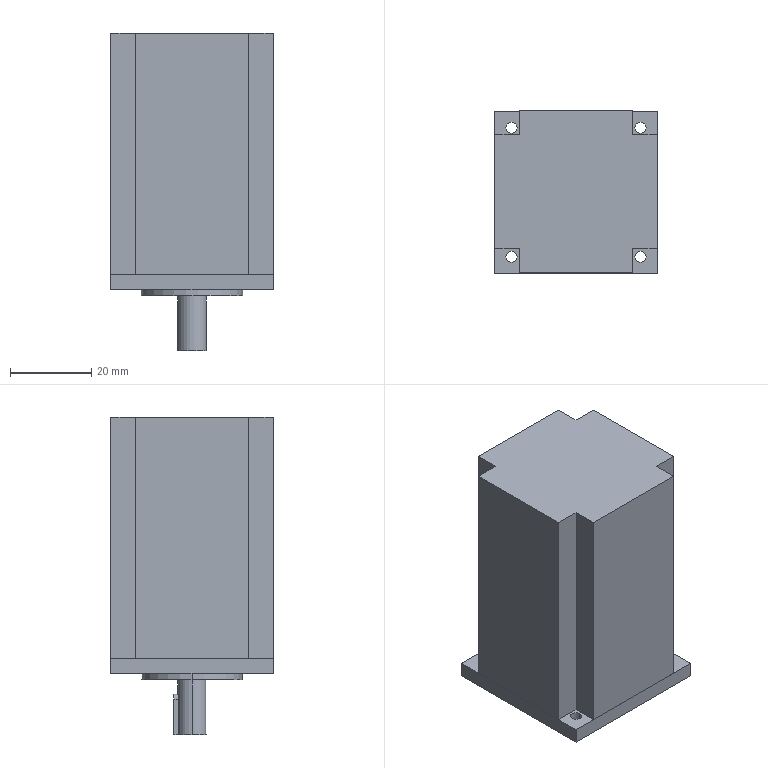Part | SolidWorks | features BaseBody 2, Scale 1 | 2 solids | 38 faces | box 40 x 40 x 78.25 mm | volume 93825 mm3 | plane 25 | cylinder 13 | commonest cylinder face diameters 2.75 x8 7 x2 25 x2 2.5 x1
STEP:
#1=CARTESIAN_POINT('',(14.535,-15.91,0.));
#2=VERTEX_POINT('',#1);
#3=CARTESIAN_POINT('',(17.285,-15.91,0.));
#4=VERTEX_POINT('',#3);
#5=CARTESIAN_POINT('',(15.91,-15.91,0.));
#6=DIRECTION('',(0.,0.,1.));
#7=DIRECTION('',(1.,0.,0.));
#8=AXIS2_PLACEMENT_3D('',#5,#6,#7);
#9=CIRCLE('',#8,1.375);
#10=EDGE_CURVE('',#2,#4,#9,.T.);
#11=ORIENTED_EDGE('',*,*,#10,.F.);
#12=CARTESIAN_POINT('',(14.535,-15.91,3.75));
#13=VERTEX_POINT('',#12);
#14=CARTESIAN_POINT('',(14.535,-15.91,3.75));
#15=DIRECTION('',(0.,0.,1.));
#16=VECTOR('',#15,1000.);
#17=LINE('',#14,#16);
#18=EDGE_CURVE('',#2,#13,#17,.T.);
#19=ORIENTED_EDGE('',*,*,#18,.T.);
#20=CARTESIAN_POINT('',(17.285,-15.91,3.75));
#21=VERTEX_POINT('',#20);
#22=CARTESIAN_POINT('',(15.91,-15.91,3.75));
#23=DIRECTION('',(0.,0.,1.));
#24=DIRECTION('',(1.,0.,0.));
#25=AXIS2_PLACEMENT_3D('',#22,#23,#24);
#26=CIRCLE('',#25,1.375);
#27=EDGE_CURVE('',#13,#21,#26,.T.);
#28=ORIENTED_EDGE('',*,*,#27,.T.);
#29=CARTESIAN_POINT('',(17.285,-15.91,3.75));
#30=DIRECTION('',(0.,0.,1.));
#31=VECTOR('',#30,1000.);
#32=LINE('',#29,#31);
#33=EDGE_CURVE('',#4,#21,#32,.T.);
#34=ORIENTED_EDGE('',*,*,#33,.F.);
#35=EDGE_LOOP('',(#11,#19,#28,#34));
#36=FACE_OUTER_BOUND('',#35,.T.);
#37=CARTESIAN_POINT('',(15.91,-15.91,3.75));
#38=DIRECTION('',(0.,0.,1.));
#39=DIRECTION('',(1.,0.,0.));
#40=AXIS2_PLACEMENT_3D('',#37,#38,#39);
#41=CYLINDRICAL_SURFACE('',#40,1.375);
#42=ADVANCED_FACE('',(#36),#41,.F.);
#43=CARTESIAN_POINT('',(-17.285,-15.91,0.));
#44=VERTEX_POINT('',#43);
#45=CARTESIAN_POINT('',(-14.535,-15.91,0.));
#46=VERTEX_POINT('',#45);
#47=CARTESIAN_POINT('',(-15.91,-15.91,0.));
#48=DIRECTION('',(0.,0.,1.));
#49=DIRECTION('',(1.,0.,0.));
#50=AXIS2_PLACEMENT_3D('',#47,#48,#49);
#51=CIRCLE('',#50,1.375);
#52=EDGE_CURVE('',#44,#46,#51,.T.);
#53=ORIENTED_EDGE('',*,*,#52,.F.);
#54=CARTESIAN_POINT('',(-17.285,-15.91,3.75));
#55=VERTEX_POINT('',#54);
#56=CARTESIAN_POINT('',(-17.285,-15.91,3.75));
#57=DIRECTION('',(0.,0.,1.));
#58=VECTOR('',#57,1000.);
#59=LINE('',#56,#58);
#60=EDGE_CURVE('',#44,#55,#59,.T.);
#61=ORIENTED_EDGE('',*,*,#60,.T.);
#62=CARTESIAN_POINT('',(-14.535,-15.91,3.75));
#63=VERTEX_POINT('',#62);
#64=CARTESIAN_POINT('',(-15.91,-15.91,3.75));
#65=DIRECTION('',(0.,0.,1.));
#66=DIRECTION('',(1.,0.,0.));
#67=AXIS2_PLACEMENT_3D('',#64,#65,#66);
#68=CIRCLE('',#67,1.375);
#69=EDGE_CURVE('',#55,#63,#68,.T.);
#70=ORIENTED_EDGE('',*,*,#69,.T.);
#71=CARTESIAN_POINT('',(-14.535,-15.91,3.75));
#72=DIRECTION('',(0.,0.,1.));
#73=VECTOR('',#72,1000.);
#74=LINE('',#71,#73);
#75=EDGE_CURVE('',#46,#63,#74,.T.);
#76=ORIENTED_EDGE('',*,*,#75,.F.);
#77=EDGE_LOOP('',(#53,#61,#70,#76));
#78=FACE_OUTER_BOUND('',#77,.T.);
#79=CARTESIAN_POINT('',(-15.91,-15.91,3.75));
#80=DIRECTION('',(0.,0.,1.));
#81=DIRECTION('',(1.,0.,0.));
#82=AXIS2_PLACEMENT_3D('',#79,#80,#81);
#83=CYLINDRICAL_SURFACE('',#82,1.375);
#84=ADVANCED_FACE('',(#78),#83,.F.);
#85=CARTESIAN_POINT('',(-17.285,15.91,0.));
#86=VERTEX_POINT('',#85);
#87=CARTESIAN_POINT('',(-14.535,15.91,0.));
#88=VERTEX_POINT('',#87);
#89=CARTESIAN_POINT('',(-15.91,15.91,0.));
#90=DIRECTION('',(0.,0.,1.));
#91=DIRECTION('',(1.,0.,0.));
#92=AXIS2_PLACEMENT_3D('',#89,#90,#91);
#93=CIRCLE('',#92,1.375);
#94=EDGE_CURVE('',#86,#88,#93,.T.);
#95=ORIENTED_EDGE('',*,*,#94,.F.);
#96=CARTESIAN_POINT('',(-17.285,15.91,3.75));
#97=VERTEX_POINT('',#96);
#98=CARTESIAN_POINT('',(-17.285,15.91,3.75));
#99=DIRECTION('',(0.,0.,1.));
#100=VECTOR('',#99,1000.);
#101=LINE('',#98,#100);
#102=EDGE_CURVE('',#86,#97,#101,.T.);
#103=ORIENTED_EDGE('',*,*,#102,.T.);
#104=CARTESIAN_POINT('',(-14.535,15.91,3.75));
#105=VERTEX_POINT('',#104);
#106=CARTESIAN_POINT('',(-15.91,15.91,3.75));
#107=DIRECTION('',(0.,0.,1.));
#108=DIRECTION('',(1.,0.,0.));
#109=AXIS2_PLACEMENT_3D('',#106,#107,#108);
#110=CIRCLE('',#109,1.375);
#111=EDGE_CURVE('',#97,#105,#110,.T.);
#112=ORIENTED_EDGE('',*,*,#111,.T.);
#113=CARTESIAN_POINT('',(-14.535,15.91,3.75));
#114=DIRECTION('',(0.,0.,1.));
#115=VECTOR('',#114,1000.);
#116=LINE('',#113,#115);
#117=EDGE_CURVE('',#88,#105,#116,.T.);
#118=ORIENTED_EDGE('',*,*,#117,.F.);
#119=EDGE_LOOP('',(#95,#103,#112,#118));
#120=FACE_OUTER_BOUND('',#119,.T.);
#121=CARTESIAN_POINT('',(-15.91,15.91,3.75));
#122=DIRECTION('',(0.,0.,1.));
#123=DIRECTION('',(1.,0.,0.));
#124=AXIS2_PLACEMENT_3D('',#121,#122,#123);
#125=CYLINDRICAL_SURFACE('',#124,1.375);
#126=ADVANCED_FACE('',(#120),#125,.F.);
#127=CARTESIAN_POINT('',(14.535,15.91,0.));
#128=VERTEX_POINT('',#127);
#129=CARTESIAN_POINT('',(17.285,15.91,0.));
#130=VERTEX_POINT('',#129);
#131=CARTESIAN_POINT('',(15.91,15.91,0.));
#132=DIRECTION('',(0.,0.,1.));
#133=DIRECTION('',(1.,0.,0.));
#134=AXIS2_PLACEMENT_3D('',#131,#132,#133);
#135=CIRCLE('',#134,1.375);
#136=EDGE_CURVE('',#128,#130,#135,.T.);
#137=ORIENTED_EDGE('',*,*,#136,.F.);
#138=CARTESIAN_POINT('',(14.535,15.91,3.75));
#139=VERTEX_POINT('',#138);
#140=CARTESIAN_POINT('',(14.535,15.91,3.75));
#141=DIRECTION('',(0.,0.,1.));
#142=VECTOR('',#141,1000.);
#143=LINE('',#140,#142);
#144=EDGE_CURVE('',#128,#139,#143,.T.);
#145=ORIENTED_EDGE('',*,*,#144,.T.);
#146=CARTESIAN_POINT('',(17.285,15.91,3.75));
#147=VERTEX_POINT('',#146);
#148=CARTESIAN_POINT('',(15.91,15.91,3.75));
#149=DIRECTION('',(0.,0.,1.));
#150=DIRECTION('',(1.,0.,0.));
#151=AXIS2_PLACEMENT_3D('',#148,#149,#150);
#152=CIRCLE('',#151,1.375);
#153=EDGE_CURVE('',#139,#147,#152,.T.);
#154=ORIENTED_EDGE('',*,*,#153,.T.);
#155=CARTESIAN_POINT('',(17.285,15.91,3.75));
#156=DIRECTION('',(0.,0.,1.));
#157=VECTOR('',#156,1000.);
#158=LINE('',#155,#157);
#159=EDGE_CURVE('',#130,#147,#158,.T.);
#160=ORIENTED_EDGE('',*,*,#159,.F.);
#161=EDGE_LOOP('',(#137,#145,#154,#160));
#162=FACE_OUTER_BOUND('',#161,.T.);
#163=CARTESIAN_POINT('',(15.91,15.91,3.75));
#164=DIRECTION('',(0.,0.,1.));
#165=DIRECTION('',(1.,0.,0.));
#166=AXIS2_PLACEMENT_3D('',#163,#164,#165);
#167=CYLINDRICAL_SURFACE('',#166,1.375);
#168=ADVANCED_FACE('',(#162),#167,.F.);
#169=CARTESIAN_POINT('',(12.5,0.,-1.5));
#170=VERTEX_POINT('',#169);
#171=CARTESIAN_POINT('',(-12.5,0.,-1.5));
#172=VERTEX_POINT('',#171);
#173=CARTESIAN_POINT('',(0.,0.,-1.5));
#174=DIRECTION('',(0.,0.,1.));
#175=DIRECTION('',(1.,0.,0.));
#176=AXIS2_PLACEMENT_3D('',#173,#174,#175);
#177=CIRCLE('',#176,12.5);
#178=EDGE_CURVE('',#170,#172,#177,.T.);
#179=ORIENTED_EDGE('',*,*,#178,.T.);
#180=CARTESIAN_POINT('',(-12.5,0.,0.));
#181=VERTEX_POINT('',#180);
#182=CARTESIAN_POINT('',(-12.5,0.,0.));
#183=DIRECTION('',(0.,0.,1.));
#184=VECTOR('',#183,1000.);
#185=LINE('',#182,#184);
#186=EDGE_CURVE('',#172,#181,#185,.T.);
#187=ORIENTED_EDGE('',*,*,#186,.T.);
#188=CARTESIAN_POINT('',(12.5,0.,0.));
#189=VERTEX_POINT('',#188);
#190=CARTESIAN_POINT('',(0.,0.,0.));
#191=DIRECTION('',(0.,0.,1.));
#192=DIRECTION('',(1.,0.,0.));
#193=AXIS2_PLACEMENT_3D('',#190,#191,#192);
#194=CIRCLE('',#193,12.5);
#195=EDGE_CURVE('',#189,#181,#194,.T.);
#196=ORIENTED_EDGE('',*,*,#195,.F.);
#197=CARTESIAN_POINT('',(12.5,0.,0.));
#198=DIRECTION('',(0.,0.,1.));
#199=VECTOR('',#198,1000.);
#200=LINE('',#197,#199);
#201=EDGE_CURVE('',#170,#189,#200,.T.);
#202=ORIENTED_EDGE('',*,*,#201,.F.);
#203=EDGE_LOOP('',(#179,#187,#196,#202));
#204=FACE_OUTER_BOUND('',#203,.T.);
#205=CARTESIAN_POINT('',(0.,0.,0.));
#206=DIRECTION('',(0.,0.,1.));
#207=DIRECTION('',(1.,0.,0.));
#208=AXIS2_PLACEMENT_3D('',#205,#206,#207);
#209=CYLINDRICAL_SURFACE('',#208,12.5);
#210=ADVANCED_FACE('',(#204),#209,.T.);
#211=CARTESIAN_POINT('',(-1.25,3.269,-15.));
#212=VERTEX_POINT('',#211);
#213=CARTESIAN_POINT('',(-3.5,0.,-15.));
#214=VERTEX_POINT('',#213);
#215=CARTESIAN_POINT('',(0.,0.,-15.));
#216=DIRECTION('',(0.,0.,1.));
#217=DIRECTION('',(1.,0.,0.));
#218=AXIS2_PLACEMENT_3D('',#215,#216,#217);
#219=CIRCLE('',#218,3.5);
#220=EDGE_CURVE('',#212,#214,#219,.T.);
#221=ORIENTED_EDGE('',*,*,#220,.T.);
#222=CARTESIAN_POINT('',(-3.5,0.,-1.5));
#223=VERTEX_POINT('',#222);
#224=CARTESIAN_POINT('',(-3.5,0.,0.));
#225=DIRECTION('',(0.,0.,1.));
#226=VECTOR('',#225,1000.);
#227=LINE('',#224,#226);
#228=EDGE_CURVE('',#214,#223,#227,.T.);
#229=ORIENTED_EDGE('',*,*,#228,.T.);
#230=CARTESIAN_POINT('',(3.5,0.,-1.5));
#231=VERTEX_POINT('',#230);
#232=CARTESIAN_POINT('',(0.,0.,-1.5));
#233=DIRECTION('',(0.,0.,-1.));
#234=DIRECTION('',(1.,0.,0.));
#235=AXIS2_PLACEMENT_3D('',#232,#233,#234);
#236=CIRCLE('',#235,3.5);
#237=EDGE_CURVE('',#223,#231,#236,.T.);
#238=ORIENTED_EDGE('',*,*,#237,.T.);
#239=CARTESIAN_POINT('',(3.5,0.,-15.));
#240=VERTEX_POINT('',#239);
#241=CARTESIAN_POINT('',(3.5,0.,0.));
#242=DIRECTION('',(0.,0.,1.));
#243=VECTOR('',#242,1000.);
#244=LINE('',#241,#243);
#245=EDGE_CURVE('',#240,#231,#244,.T.);
#246=ORIENTED_EDGE('',*,*,#245,.F.);
#247=CARTESIAN_POINT('',(1.25,3.269,-15.));
#248=VERTEX_POINT('',#247);
#249=CARTESIAN_POINT('',(0.,0.,-15.));
#250=DIRECTION('',(0.,0.,1.));
#251=DIRECTION('',(1.,0.,0.));
#252=AXIS2_PLACEMENT_3D('',#249,#250,#251);
#253=CIRCLE('',#252,3.5);
#254=EDGE_CURVE('',#240,#248,#253,.T.);
#255=ORIENTED_EDGE('',*,*,#254,.T.);
#256=CARTESIAN_POINT('',(1.25,3.269,-6.25));
#257=VERTEX_POINT('',#256);
#258=CARTESIAN_POINT('',(1.25,3.269,0.));
#259=DIRECTION('',(0.,0.,1.));
#260=VECTOR('',#259,1000.);
#261=LINE('',#258,#260);
#262=EDGE_CURVE('',#248,#257,#261,.T.);
#263=ORIENTED_EDGE('',*,*,#262,.T.);
#264=CARTESIAN_POINT('',(-1.25,3.269,-6.25));
#265=VERTEX_POINT('',#264);
#266=CARTESIAN_POINT('',(1.25,3.269,-6.25));
#267=CARTESIAN_POINT('',(1.25,3.269,-6.083));
#268=CARTESIAN_POINT('',(1.217,3.282,-5.92));
#269=CARTESIAN_POINT('',(1.091,3.326,-5.618));
#270=CARTESIAN_POINT('',(0.9983,3.357,-5.481));
#271=CARTESIAN_POINT('',(0.7698,3.416,-5.252));
#272=CARTESIAN_POINT('',(0.6316,3.446,-5.159));
#273=CARTESIAN_POINT('',(0.3313,3.488,-5.034));
#274=CARTESIAN_POINT('',(0.166,3.5,-5.));
#275=CARTESIAN_POINT('',(-0.0809,3.5,-5.));
#276=CARTESIAN_POINT('',(-0.1645,3.497,-5.008));
#277=CARTESIAN_POINT('',(-0.3254,3.486,-5.04));
#278=CARTESIAN_POINT('',(-0.4037,3.477,-5.064));
#279=CARTESIAN_POINT('',(-0.6321,3.446,-5.159));
#280=CARTESIAN_POINT('',(-0.7689,3.417,-5.251));
#281=CARTESIAN_POINT('',(-0.9411,3.372,-5.423));
#282=CARTESIAN_POINT('',(-0.9924,3.357,-5.486));
#283=CARTESIAN_POINT('',(-1.083,3.329,-5.621));
#284=CARTESIAN_POINT('',(-1.122,3.315,-5.693));
#285=CARTESIAN_POINT('',(-1.216,3.283,-5.919));
#286=CARTESIAN_POINT('',(-1.25,3.269,-6.083));
#287=CARTESIAN_POINT('',(-1.25,3.269,-6.25));
#288=B_SPLINE_CURVE_WITH_KNOTS('',3,(#266,#267,#268,#269,#270,#271,#272,#273,#274,#275,#276,#277,#278,#279,#280,#281,#282,#283,#284,#285,#286,#287),.UNSPECIFIED.,.F.,.F.,(4,2,2,2,2,2,2,2,2,2,4),(0.,0.0004924,0.0009848,0.001477,0.00197,0.002216,0.002462,0.002954,0.003201,0.003447,0.003939),.UNSPECIFIED.);
#289=EDGE_CURVE('',#257,#265,#288,.T.);
#290=ORIENTED_EDGE('',*,*,#289,.T.);
#291=CARTESIAN_POINT('',(-1.25,3.269,0.));
#292=DIRECTION('',(0.,0.,-1.));
#293=VECTOR('',#292,1000.);
#294=LINE('',#291,#293);
#295=EDGE_CURVE('',#265,#212,#294,.T.);
#296=ORIENTED_EDGE('',*,*,#295,.T.);
#297=EDGE_LOOP('',(#221,#229,#238,#246,#255,#263,#290,#296));
#298=FACE_OUTER_BOUND('',#297,.T.);
#299=CARTESIAN_POINT('',(0.,0.,0.));
#300=DIRECTION('',(0.,0.,1.));
#301=DIRECTION('',(1.,0.,0.));
#302=AXIS2_PLACEMENT_3D('',#299,#300,#301);
#303=CYLINDRICAL_SURFACE('',#302,3.5);
#304=ADVANCED_FACE('',(#298),#303,.T.);
#305=CARTESIAN_POINT('',(15.91,-15.91,3.75));
#306=DIRECTION('',(0.,0.,1.));
#307=DIRECTION('',(1.,0.,0.));
#308=AXIS2_PLACEMENT_3D('',#305,#306,#307);
#309=CIRCLE('',#308,1.375);
#310=EDGE_CURVE('',#21,#13,#309,.T.);
#311=ORIENTED_EDGE('',*,*,#310,.F.);
#312=ORIENTED_EDGE('',*,*,#27,.F.);
#313=EDGE_LOOP('',(#311,#312));
#314=FACE_BOUND('',#313,.T.);
#315=CARTESIAN_POINT('',(-15.91,-15.91,3.75));
#316=DIRECTION('',(0.,0.,1.));
#317=DIRECTION('',(1.,0.,0.));
#318=AXIS2_PLACEMENT_3D('',#315,#316,#317);
#319=CIRCLE('',#318,1.375);
#320=EDGE_CURVE('',#63,#55,#319,.T.);
#321=ORIENTED_EDGE('',*,*,#320,.F.);
#322=ORIENTED_EDGE('',*,*,#69,.F.);
#323=EDGE_LOOP('',(#321,#322));
#324=FACE_BOUND('',#323,.T.);
#325=CARTESIAN_POINT('',(-15.91,15.91,3.75));
#326=DIRECTION('',(0.,0.,1.));
#327=DIRECTION('',(1.,0.,0.));
#328=AXIS2_PLACEMENT_3D('',#325,#326,#327);
#329=CIRCLE('',#328,1.375);
#330=EDGE_CURVE('',#105,#97,#329,.T.);
#331=ORIENTED_EDGE('',*,*,#330,.F.);
#332=ORIENTED_EDGE('',*,*,#111,.F.);
#333=EDGE_LOOP('',(#331,#332));
#334=FACE_BOUND('',#333,.T.);
#335=CARTESIAN_POINT('',(15.91,15.91,3.75));
#336=DIRECTION('',(0.,0.,1.));
#337=DIRECTION('',(1.,0.,0.));
#338=AXIS2_PLACEMENT_3D('',#335,#336,#337);
#339=CIRCLE('',#338,1.375);
#340=EDGE_CURVE('',#147,#139,#339,.T.);
#341=ORIENTED_EDGE('',*,*,#340,.F.);
#342=ORIENTED_EDGE('',*,*,#153,.F.);
#343=EDGE_LOOP('',(#341,#342));
#344=FACE_BOUND('',#343,.T.);
#345=CARTESIAN_POINT('',(-20.,20.,3.75));
#346=VERTEX_POINT('',#345);
#347=CARTESIAN_POINT('',(20.,20.,3.75));
#348=VERTEX_POINT('',#347);
#349=CARTESIAN_POINT('',(20.,20.,3.75));
#350=DIRECTION('',(1.,0.,0.));
#351=VECTOR('',#350,1000.);
#352=LINE('',#349,#351);
#353=EDGE_CURVE('',#346,#348,#352,.T.);
#354=ORIENTED_EDGE('',*,*,#353,.F.);
#355=CARTESIAN_POINT('',(-20.,-20.,3.75));
#356=VERTEX_POINT('',#355);
#357=CARTESIAN_POINT('',(-20.,20.,3.75));
#358=DIRECTION('',(0.,1.,0.));
#359=VECTOR('',#358,1000.);
#360=LINE('',#357,#359);
#361=EDGE_CURVE('',#356,#346,#360,.T.);
#362=ORIENTED_EDGE('',*,*,#361,.F.);
#363=CARTESIAN_POINT('',(20.,-20.,3.75));
#364=VERTEX_POINT('',#363);
#365=CARTESIAN_POINT('',(20.,-20.,3.75));
#366=DIRECTION('',(-1.,0.,0.));
#367=VECTOR('',#366,1000.);
#368=LINE('',#365,#367);
#369=EDGE_CURVE('',#364,#356,#368,.T.);
#370=ORIENTED_EDGE('',*,*,#369,.F.);
#371=CARTESIAN_POINT('',(20.,20.,3.75));
#372=DIRECTION('',(0.,-1.,0.));
#373=VECTOR('',#372,1000.);
#374=LINE('',#371,#373);
#375=EDGE_CURVE('',#348,#364,#374,.T.);
#376=ORIENTED_EDGE('',*,*,#375,.F.);
#377=EDGE_LOOP('',(#354,#362,#370,#376));
#378=FACE_OUTER_BOUND('',#377,.T.);
#379=CARTESIAN_POINT('',(20.,20.,3.75));
#380=DIRECTION('',(0.,0.,-1.));
#381=DIRECTION('',(-1.,0.,0.));
#382=AXIS2_PLACEMENT_3D('',#379,#380,#381);
#383=PLANE('',#382);
#384=ADVANCED_FACE('',(#314,#324,#334,#344,#378),#383,.F.);
#385=ORIENTED_EDGE('',*,*,#18,.F.);
#386=CARTESIAN_POINT('',(15.91,-15.91,0.));
#387=DIRECTION('',(0.,0.,1.));
#388=DIRECTION('',(1.,0.,0.));
#389=AXIS2_PLACEMENT_3D('',#386,#387,#388);
#390=CIRCLE('',#389,1.375);
#391=EDGE_CURVE('',#4,#2,#390,.T.);
#392=ORIENTED_EDGE('',*,*,#391,.F.);
#393=ORIENTED_EDGE('',*,*,#33,.T.);
#394=ORIENTED_EDGE('',*,*,#310,.T.);
#395=EDGE_LOOP('',(#385,#392,#393,#394));
#396=FACE_OUTER_BOUND('',#395,.T.);
#397=CARTESIAN_POINT('',(15.91,-15.91,3.75));
#398=DIRECTION('',(0.,0.,1.));
#399=DIRECTION('',(1.,0.,0.));
#400=AXIS2_PLACEMENT_3D('',#397,#398,#399);
#401=CYLINDRICAL_SURFACE('',#400,1.375);
#402=ADVANCED_FACE('',(#396),#401,.F.);
#403=ORIENTED_EDGE('',*,*,#60,.F.);
#404=CARTESIAN_POINT('',(-15.91,-15.91,0.));
#405=DIRECTION('',(0.,0.,1.));
#406=DIRECTION('',(1.,0.,0.));
#407=AXIS2_PLACEMENT_3D('',#404,#405,#406);
#408=CIRCLE('',#407,1.375);
#409=EDGE_CURVE('',#46,#44,#408,.T.);
#410=ORIENTED_EDGE('',*,*,#409,.F.);
#411=ORIENTED_EDGE('',*,*,#75,.T.);
#412=ORIENTED_EDGE('',*,*,#320,.T.);
#413=EDGE_LOOP('',(#403,#410,#411,#412));
#414=FACE_OUTER_BOUND('',#413,.T.);
#415=CARTESIAN_POINT('',(-15.91,-15.91,3.75));
#416=DIRECTION('',(0.,0.,1.));
#417=DIRECTION('',(1.,0.,0.));
#418=AXIS2_PLACEMENT_3D('',#415,#416,#417);
#419=CYLINDRICAL_SURFACE('',#418,1.375);
#420=ADVANCED_FACE('',(#414),#419,.F.);
#421=ORIENTED_EDGE('',*,*,#102,.F.);
#422=CARTESIAN_POINT('',(-15.91,15.91,0.));
#423=DIRECTION('',(0.,0.,1.));
#424=DIRECTION('',(1.,0.,0.));
#425=AXIS2_PLACEMENT_3D('',#422,#423,#424);
#426=CIRCLE('',#425,1.375);
#427=EDGE_CURVE('',#88,#86,#426,.T.);
#428=ORIENTED_EDGE('',*,*,#427,.F.);
#429=ORIENTED_EDGE('',*,*,#117,.T.);
#430=ORIENTED_EDGE('',*,*,#330,.T.);
#431=EDGE_LOOP('',(#421,#428,#429,#430));
#432=FACE_OUTER_BOUND('',#431,.T.);
#433=CARTESIAN_POINT('',(-15.91,15.91,3.75));
#434=DIRECTION('',(0.,0.,1.));
#435=DIRECTION('',(1.,0.,0.));
#436=AXIS2_PLACEMENT_3D('',#433,#434,#435);
#437=CYLINDRICAL_SURFACE('',#436,1.375);
#438=ADVANCED_FACE('',(#432),#437,.F.);
#439=ORIENTED_EDGE('',*,*,#144,.F.);
#440=CARTESIAN_POINT('',(15.91,15.91,0.));
#441=DIRECTION('',(0.,0.,1.));
#442=DIRECTION('',(1.,0.,0.));
#443=AXIS2_PLACEMENT_3D('',#440,#441,#442);
#444=CIRCLE('',#443,1.375);
#445=EDGE_CURVE('',#130,#128,#444,.T.);
#446=ORIENTED_EDGE('',*,*,#445,.F.);
#447=ORIENTED_EDGE('',*,*,#159,.T.);
#448=ORIENTED_EDGE('',*,*,#340,.T.);
#449=EDGE_LOOP('',(#439,#446,#447,#448));
#450=FACE_OUTER_BOUND('',#449,.T.);
#451=CARTESIAN_POINT('',(15.91,15.91,3.75));
#452=DIRECTION('',(0.,0.,1.));
#453=DIRECTION('',(1.,0.,0.));
#454=AXIS2_PLACEMENT_3D('',#451,#452,#453);
#455=CYLINDRICAL_SURFACE('',#454,1.375);
#456=ADVANCED_FACE('',(#450),#455,.F.);
#457=CARTESIAN_POINT('',(20.,20.,0.));
#458=VERTEX_POINT('',#457);
#459=CARTESIAN_POINT('',(20.,20.,3.75));
#460=DIRECTION('',(0.,0.,-1.));
#461=VECTOR('',#460,1000.);
#462=LINE('',#459,#461);
#463=EDGE_CURVE('',#348,#458,#462,.T.);
#464=ORIENTED_EDGE('',*,*,#463,.F.);
#465=ORIENTED_EDGE('',*,*,#375,.T.);
#466=CARTESIAN_POINT('',(20.,-20.,0.));
#467=VERTEX_POINT('',#466);
#468=CARTESIAN_POINT('',(20.,-20.,3.75));
#469=DIRECTION('',(0.,0.,1.));
#470=VECTOR('',#469,1000.);
#471=LINE('',#468,#470);
#472=EDGE_CURVE('',#467,#364,#471,.T.);
#473=ORIENTED_EDGE('',*,*,#472,.F.);
#474=CARTESIAN_POINT('',(20.,-20.,0.));
#475=DIRECTION('',(0.,-1.,0.));
#476=VECTOR('',#475,1000.);
#477=LINE('',#474,#476);
#478=EDGE_CURVE('',#458,#467,#477,.T.);
#479=ORIENTED_EDGE('',*,*,#478,.F.);
#480=EDGE_LOOP('',(#464,#465,#473,#479));
#481=FACE_OUTER_BOUND('',#480,.T.);
#482=CARTESIAN_POINT('',(20.,-20.,3.75));
#483=DIRECTION('',(-1.,0.,0.));
#484=DIRECTION('',(0.,0.,1.));
#485=AXIS2_PLACEMENT_3D('',#482,#483,#484);
#486=PLANE('',#485);
#487=ADVANCED_FACE('',(#481),#486,.F.);
#488=CARTESIAN_POINT('',(-20.,20.,0.));
#489=VERTEX_POINT('',#488);
#490=CARTESIAN_POINT('',(-20.,20.,3.75));
#491=DIRECTION('',(0.,0.,-1.));
#492=VECTOR('',#491,1000.);
#493=LINE('',#490,#492);
#494=EDGE_CURVE('',#346,#489,#493,.T.);
#495=ORIENTED_EDGE('',*,*,#494,.F.);
#496=ORIENTED_EDGE('',*,*,#353,.T.);
#497=ORIENTED_EDGE('',*,*,#463,.T.);
#498=CARTESIAN_POINT('',(-20.,20.,0.));
#499=DIRECTION('',(1.,0.,0.));
#500=VECTOR('',#499,1000.);
#501=LINE('',#498,#500);
#502=EDGE_CURVE('',#489,#458,#501,.T.);
#503=ORIENTED_EDGE('',*,*,#502,.F.);
#504=EDGE_LOOP('',(#495,#496,#497,#503));
#505=FACE_OUTER_BOUND('',#504,.T.);
#506=CARTESIAN_POINT('',(-20.,20.,3.75));
#507=DIRECTION('',(0.,-1.,0.));
#508=DIRECTION('',(0.,0.,-1.));
#509=AXIS2_PLACEMENT_3D('',#506,#507,#508);
#510=PLANE('',#509);
#511=ADVANCED_FACE('',(#505),#510,.F.);
#512=CARTESIAN_POINT('',(-20.,-20.,0.));
#513=VERTEX_POINT('',#512);
#514=CARTESIAN_POINT('',(-20.,-20.,3.75));
#515=DIRECTION('',(0.,0.,-1.));
#516=VECTOR('',#515,1000.);
#517=LINE('',#514,#516);
#518=EDGE_CURVE('',#356,#513,#517,.T.);
#519=ORIENTED_EDGE('',*,*,#518,.F.);
#520=ORIENTED_EDGE('',*,*,#361,.T.);
#521=ORIENTED_EDGE('',*,*,#494,.T.);
#522=CARTESIAN_POINT('',(-20.,-20.,0.));
#523=DIRECTION('',(0.,1.,0.));
#524=VECTOR('',#523,1000.);
#525=LINE('',#522,#524);
#526=EDGE_CURVE('',#513,#489,#525,.T.);
#527=ORIENTED_EDGE('',*,*,#526,.F.);
#528=EDGE_LOOP('',(#519,#520,#521,#527));
#529=FACE_OUTER_BOUND('',#528,.T.);
#530=CARTESIAN_POINT('',(-20.,-20.,3.75));
#531=DIRECTION('',(1.,0.,0.));
#532=DIRECTION('',(0.,0.,-1.));
#533=AXIS2_PLACEMENT_3D('',#530,#531,#532);
#534=PLANE('',#533);
#535=ADVANCED_FACE('',(#529),#534,.F.);
#536=ORIENTED_EDGE('',*,*,#472,.T.);
#537=ORIENTED_EDGE('',*,*,#369,.T.);
#538=ORIENTED_EDGE('',*,*,#518,.T.);
#539=CARTESIAN_POINT('',(-20.,-20.,0.));
#540=DIRECTION('',(-1.,0.,0.));
#541=VECTOR('',#540,1000.);
#542=LINE('',#539,#541);
#543=EDGE_CURVE('',#467,#513,#542,.T.);
#544=ORIENTED_EDGE('',*,*,#543,.F.);
#545=EDGE_LOOP('',(#536,#537,#538,#544));
#546=FACE_OUTER_BOUND('',#545,.T.);
#547=CARTESIAN_POINT('',(-20.,-20.,3.75));
#548=DIRECTION('',(0.,1.,0.));
#549=DIRECTION('',(0.,0.,1.));
#550=AXIS2_PLACEMENT_3D('',#547,#548,#549);
#551=PLANE('',#550);
#552=ADVANCED_FACE('',(#546),#551,.F.);
#553=ORIENTED_EDGE('',*,*,#391,.T.);
#554=ORIENTED_EDGE('',*,*,#10,.T.);
#555=EDGE_LOOP('',(#553,#554));
#556=FACE_BOUND('',#555,.T.);
#557=ORIENTED_EDGE('',*,*,#409,.T.);
#558=ORIENTED_EDGE('',*,*,#52,.T.);
#559=EDGE_LOOP('',(#557,#558));
#560=FACE_BOUND('',#559,.T.);
#561=ORIENTED_EDGE('',*,*,#427,.T.);
#562=ORIENTED_EDGE('',*,*,#94,.T.);
#563=EDGE_LOOP('',(#561,#562));
#564=FACE_BOUND('',#563,.T.);
#565=ORIENTED_EDGE('',*,*,#445,.T.);
#566=ORIENTED_EDGE('',*,*,#136,.T.);
#567=EDGE_LOOP('',(#565,#566));
#568=FACE_BOUND('',#567,.T.);
#569=ORIENTED_EDGE('',*,*,#195,.T.);
#570=CARTESIAN_POINT('',(0.,0.,0.));
#571=DIRECTION('',(0.,0.,1.));
#572=DIRECTION('',(1.,0.,0.));
#573=AXIS2_PLACEMENT_3D('',#570,#571,#572);
#574=CIRCLE('',#573,12.5);
#575=EDGE_CURVE('',#181,#189,#574,.T.);
#576=ORIENTED_EDGE('',*,*,#575,.T.);
#577=EDGE_LOOP('',(#569,#576));
#578=FACE_BOUND('',#577,.T.);
#579=ORIENTED_EDGE('',*,*,#526,.T.);
#580=ORIENTED_EDGE('',*,*,#502,.T.);
#581=ORIENTED_EDGE('',*,*,#478,.T.);
#582=ORIENTED_EDGE('',*,*,#543,.T.);
#583=EDGE_LOOP('',(#579,#580,#581,#582));
#584=FACE_OUTER_BOUND('',#583,.T.);
#585=CARTESIAN_POINT('',(20.,20.,0.));
#586=DIRECTION('',(0.,0.,-1.));
#587=DIRECTION('',(-1.,0.,0.));
#588=AXIS2_PLACEMENT_3D('',#585,#586,#587);
#589=PLANE('',#588);
#590=ADVANCED_FACE('',(#556,#560,#564,#568,#578,#584),#589,.T.);
#591=ORIENTED_EDGE('',*,*,#186,.F.);
#592=CARTESIAN_POINT('',(0.,0.,-1.5));
#593=DIRECTION('',(0.,0.,1.));
#594=DIRECTION('',(1.,0.,0.));
#595=AXIS2_PLACEMENT_3D('',#592,#593,#594);
#596=CIRCLE('',#595,12.5);
#597=EDGE_CURVE('',#172,#170,#596,.T.);
#598=ORIENTED_EDGE('',*,*,#597,.T.);
#599=ORIENTED_EDGE('',*,*,#201,.T.);
#600=ORIENTED_EDGE('',*,*,#575,.F.);
#601=EDGE_LOOP('',(#591,#598,#599,#600));
#602=FACE_OUTER_BOUND('',#601,.T.);
#603=CARTESIAN_POINT('',(0.,0.,0.));
#604=DIRECTION('',(0.,0.,1.));
#605=DIRECTION('',(1.,0.,0.));
#606=AXIS2_PLACEMENT_3D('',#603,#604,#605);
#607=CYLINDRICAL_SURFACE('',#606,12.5);
#608=ADVANCED_FACE('',(#602),#607,.T.);
#609=CARTESIAN_POINT('',(0.,0.,-1.5));
#610=DIRECTION('',(0.,0.,-1.));
#611=DIRECTION('',(1.,0.,0.));
#612=AXIS2_PLACEMENT_3D('',#609,#610,#611);
#613=CIRCLE('',#612,3.5);
#614=EDGE_CURVE('',#231,#223,#613,.T.);
#615=ORIENTED_EDGE('',*,*,#614,.F.);
#616=ORIENTED_EDGE('',*,*,#237,.F.);
#617=EDGE_LOOP('',(#615,#616));
#618=FACE_BOUND('',#617,.T.);
#619=ORIENTED_EDGE('',*,*,#178,.F.);
#620=ORIENTED_EDGE('',*,*,#597,.F.);
#621=EDGE_LOOP('',(#619,#620));
#622=FACE_OUTER_BOUND('',#621,.T.);
#623=CARTESIAN_POINT('',(0.,3.5,-1.5));
#624=DIRECTION('',(0.,0.,1.));
#625=DIRECTION('',(1.,0.,0.));
#626=AXIS2_PLACEMENT_3D('',#623,#624,#625);
#627=PLANE('',#626);
#628=ADVANCED_FACE('',(#618,#622),#627,.F.);
#629=ORIENTED_EDGE('',*,*,#228,.F.);
#630=CARTESIAN_POINT('',(0.,0.,-15.));
#631=DIRECTION('',(0.,0.,1.));
#632=DIRECTION('',(1.,0.,0.));
#633=AXIS2_PLACEMENT_3D('',#630,#631,#632);
#634=CIRCLE('',#633,3.5);
#635=EDGE_CURVE('',#214,#240,#634,.T.);
#636=ORIENTED_EDGE('',*,*,#635,.T.);
#637=ORIENTED_EDGE('',*,*,#245,.T.);
#638=ORIENTED_EDGE('',*,*,#614,.T.);
#639=EDGE_LOOP('',(#629,#636,#637,#638));
#640=FACE_OUTER_BOUND('',#639,.T.);
#641=CARTESIAN_POINT('',(0.,0.,0.));
#642=DIRECTION('',(0.,0.,1.));
#643=DIRECTION('',(1.,0.,0.));
#644=AXIS2_PLACEMENT_3D('',#641,#642,#643);
#645=CYLINDRICAL_SURFACE('',#644,3.5);
#646=ADVANCED_FACE('',(#640),#645,.T.);
#647=CARTESIAN_POINT('',(1.25,4.5,-15.));
#648=VERTEX_POINT('',#647);
#649=CARTESIAN_POINT('',(1.25,0.,-15.));
#650=DIRECTION('',(0.,1.,0.));
#651=VECTOR('',#650,1000.);
#652=LINE('',#649,#651);
#653=EDGE_CURVE('',#248,#648,#652,.T.);
#654=ORIENTED_EDGE('',*,*,#653,.F.);
#655=ORIENTED_EDGE('',*,*,#254,.F.);
#656=ORIENTED_EDGE('',*,*,#635,.F.);
#657=ORIENTED_EDGE('',*,*,#220,.F.);
#658=CARTESIAN_POINT('',(-1.25,4.5,-15.));
#659=VERTEX_POINT('',#658);
#660=CARTESIAN_POINT('',(-1.25,0.,-15.));
#661=DIRECTION('',(0.,-1.,0.));
#662=VECTOR('',#661,1000.);
#663=LINE('',#660,#662);
#664=EDGE_CURVE('',#659,#212,#663,.T.);
#665=ORIENTED_EDGE('',*,*,#664,.F.);
#666=CARTESIAN_POINT('',(0.,4.5,-15.));
#667=DIRECTION('',(-1.,0.,0.));
#668=VECTOR('',#667,1000.);
#669=LINE('',#666,#668);
#670=EDGE_CURVE('',#648,#659,#669,.T.);
#671=ORIENTED_EDGE('',*,*,#670,.F.);
#672=EDGE_LOOP('',(#654,#655,#656,#657,#665,#671));
#673=FACE_OUTER_BOUND('',#672,.T.);
#674=CARTESIAN_POINT('',(0.,0.,-15.));
#675=DIRECTION('',(0.,0.,1.));
#676=DIRECTION('',(1.,0.,0.));
#677=AXIS2_PLACEMENT_3D('',#674,#675,#676);
#678=PLANE('',#677);
#679=ADVANCED_FACE('',(#673),#678,.F.);
#680=CARTESIAN_POINT('',(-1.25,4.5,-6.25));
#681=VERTEX_POINT('',#680);
#682=CARTESIAN_POINT('',(-1.25,4.5,-5.));
#683=DIRECTION('',(0.,0.,-1.));
#684=VECTOR('',#683,1000.);
#685=LINE('',#682,#684);
#686=EDGE_CURVE('',#681,#659,#685,.T.);
#687=ORIENTED_EDGE('',*,*,#686,.T.);
#688=ORIENTED_EDGE('',*,*,#664,.T.);
#689=ORIENTED_EDGE('',*,*,#295,.F.);
#690=CARTESIAN_POINT('',(-1.25,2.,-6.25));
#691=DIRECTION('',(0.,1.,0.));
#692=VECTOR('',#691,1000.);
#693=LINE('',#690,#692);
#694=EDGE_CURVE('',#265,#681,#693,.T.);
#695=ORIENTED_EDGE('',*,*,#694,.T.);
#696=EDGE_LOOP('',(#687,#688,#689,#695));
#697=FACE_OUTER_BOUND('',#696,.T.);
#698=CARTESIAN_POINT('',(-1.25,2.,-5.));
#699=DIRECTION('',(-1.,0.,0.));
#700=DIRECTION('',(0.,0.,1.));
#701=AXIS2_PLACEMENT_3D('',#698,#699,#700);
#702=PLANE('',#701);
#703=ADVANCED_FACE('',(#697),#702,.T.);
#704=ORIENTED_EDGE('',*,*,#694,.F.);
#705=ORIENTED_EDGE('',*,*,#289,.F.);
#706=CARTESIAN_POINT('',(1.25,4.5,-6.25));
#707=VERTEX_POINT('',#706);
#708=CARTESIAN_POINT('',(1.25,4.5,-6.25));
#709=DIRECTION('',(0.,1.,0.));
#710=VECTOR('',#709,1000.);
#711=LINE('',#708,#710);
#712=EDGE_CURVE('',#257,#707,#711,.T.);
#713=ORIENTED_EDGE('',*,*,#712,.T.);
#714=CARTESIAN_POINT('',(0.,4.5,-6.25));
#715=DIRECTION('',(0.,-1.,0.));
#716=DIRECTION('',(1.,0.,0.));
#717=AXIS2_PLACEMENT_3D('',#714,#715,#716);
#718=CIRCLE('',#717,1.25);
#719=EDGE_CURVE('',#707,#681,#718,.T.);
#720=ORIENTED_EDGE('',*,*,#719,.T.);
#721=EDGE_LOOP('',(#704,#705,#713,#720));
#722=FACE_OUTER_BOUND('',#721,.T.);
#723=CARTESIAN_POINT('',(0.,4.5,-6.25));
#724=DIRECTION('',(0.,-1.,0.));
#725=DIRECTION('',(1.,0.,0.));
#726=AXIS2_PLACEMENT_3D('',#723,#724,#725);
#727=CYLINDRICAL_SURFACE('',#726,1.25);
#728=ADVANCED_FACE('',(#722),#727,.T.);
#729=ORIENTED_EDGE('',*,*,#262,.F.);
#730=ORIENTED_EDGE('',*,*,#653,.T.);
#731=CARTESIAN_POINT('',(1.25,4.5,-5.));
#732=DIRECTION('',(0.,0.,1.));
#733=VECTOR('',#732,1000.);
#734=LINE('',#731,#733);
#735=EDGE_CURVE('',#648,#707,#734,.T.);
#736=ORIENTED_EDGE('',*,*,#735,.T.);
#737=ORIENTED_EDGE('',*,*,#712,.F.);
#738=EDGE_LOOP('',(#729,#730,#736,#737));
#739=FACE_OUTER_BOUND('',#738,.T.);
#740=CARTESIAN_POINT('',(1.25,2.,-5.));
#741=DIRECTION('',(1.,0.,0.));
#742=DIRECTION('',(0.,1.,0.));
#743=AXIS2_PLACEMENT_3D('',#740,#741,#742);
#744=PLANE('',#743);
#745=ADVANCED_FACE('',(#739),#744,.T.);
#746=ORIENTED_EDGE('',*,*,#735,.F.);
#747=ORIENTED_EDGE('',*,*,#670,.T.);
#748=ORIENTED_EDGE('',*,*,#686,.F.);
#749=ORIENTED_EDGE('',*,*,#719,.F.);
#750=EDGE_LOOP('',(#746,#747,#748,#749));
#751=FACE_OUTER_BOUND('',#750,.T.);
#752=CARTESIAN_POINT('',(1.25,4.5,-5.));
#753=DIRECTION('',(0.,1.,0.));
#754=DIRECTION('',(0.,0.,1.));
#755=AXIS2_PLACEMENT_3D('',#752,#753,#754);
#756=PLANE('',#755);
#757=ADVANCED_FACE('',(#751),#756,.T.);
#758=CLOSED_SHELL('',(#42,#84,#126,#168,#210,#304,#384,#402,#420,#438,#456,#487,#511,#535,#552,#590,#608,#628,#646,#679,#703,#728,#745,#757));
#759=MANIFOLD_SOLID_BREP('',#758);
#760=CARTESIAN_POINT('',(-20.,-14.,3.75));
#761=VERTEX_POINT('',#760);
#762=CARTESIAN_POINT('',(-20.,-14.,63.25));
#763=VERTEX_POINT('',#762);
#764=CARTESIAN_POINT('',(-20.,-14.,63.25));
#765=DIRECTION('',(0.,0.,1.));
#766=VECTOR('',#765,1000.);
#767=LINE('',#764,#766);
#768=EDGE_CURVE('',#761,#763,#767,.T.);
#769=ORIENTED_EDGE('',*,*,#768,.T.);
#770=CARTESIAN_POINT('',(-20.,14.,63.25));
#771=VERTEX_POINT('',#770);
#772=CARTESIAN_POINT('',(-20.,-20.,63.25));
#773=DIRECTION('',(0.,1.,0.));
#774=VECTOR('',#773,1000.);
#775=LINE('',#772,#774);
#776=EDGE_CURVE('',#763,#771,#775,.T.);
#777=ORIENTED_EDGE('',*,*,#776,.T.);
#778=CARTESIAN_POINT('',(-20.,14.,3.75));
#779=VERTEX_POINT('',#778);
#780=CARTESIAN_POINT('',(-20.,14.,63.25));
#781=DIRECTION('',(0.,0.,-1.));
#782=VECTOR('',#781,1000.);
#783=LINE('',#780,#782);
#784=EDGE_CURVE('',#771,#779,#783,.T.);
#785=ORIENTED_EDGE('',*,*,#784,.T.);
#786=CARTESIAN_POINT('',(-20.,-20.,3.75));
#787=DIRECTION('',(0.,-1.,0.));
#788=VECTOR('',#787,1000.);
#789=LINE('',#786,#788);
#790=EDGE_CURVE('',#779,#761,#789,.T.);
#791=ORIENTED_EDGE('',*,*,#790,.T.);
#792=EDGE_LOOP('',(#769,#777,#785,#791));
#793=FACE_OUTER_BOUND('',#792,.T.);
#794=CARTESIAN_POINT('',(-20.,-20.,63.25));
#795=DIRECTION('',(-1.,0.,0.));
#796=DIRECTION('',(0.,0.,1.));
#797=AXIS2_PLACEMENT_3D('',#794,#795,#796);
#798=PLANE('',#797);
#799=ADVANCED_FACE('',(#793),#798,.T.);
#800=CARTESIAN_POINT('',(14.,14.,63.25));
#801=VERTEX_POINT('',#800);
#802=CARTESIAN_POINT('',(14.,20.,63.25));
#803=VERTEX_POINT('',#802);
#804=CARTESIAN_POINT('',(14.,20.,63.25));
#805=DIRECTION('',(0.,1.,0.));
#806=VECTOR('',#805,1000.);
#807=LINE('',#804,#806);
#808=EDGE_CURVE('',#801,#803,#807,.T.);
#809=ORIENTED_EDGE('',*,*,#808,.T.);
#810=CARTESIAN_POINT('',(-14.,20.,63.25));
#811=VERTEX_POINT('',#810);
#812=CARTESIAN_POINT('',(-20.,20.,63.25));
#813=DIRECTION('',(-1.,0.,0.));
#814=VECTOR('',#813,1000.);
#815=LINE('',#812,#814);
#816=EDGE_CURVE('',#803,#811,#815,.T.);
#817=ORIENTED_EDGE('',*,*,#816,.T.);
#818=CARTESIAN_POINT('',(-14.,14.,63.25));
#819=VERTEX_POINT('',#818);
#820=CARTESIAN_POINT('',(-14.,20.,63.25));
#821=DIRECTION('',(0.,-1.,0.));
#822=VECTOR('',#821,1000.);
#823=LINE('',#820,#822);
#824=EDGE_CURVE('',#811,#819,#823,.T.);
#825=ORIENTED_EDGE('',*,*,#824,.T.);
#826=CARTESIAN_POINT('',(-20.,14.,63.25));
#827=DIRECTION('',(-1.,0.,0.));
#828=VECTOR('',#827,1000.);
#829=LINE('',#826,#828);
#830=EDGE_CURVE('',#819,#771,#829,.T.);
#831=ORIENTED_EDGE('',*,*,#830,.T.);
#832=ORIENTED_EDGE('',*,*,#776,.F.);
#833=CARTESIAN_POINT('',(-14.,-14.,63.25));
#834=VERTEX_POINT('',#833);
#835=CARTESIAN_POINT('',(-20.,-14.,63.25));
#836=DIRECTION('',(1.,0.,0.));
#837=VECTOR('',#836,1000.);
#838=LINE('',#835,#837);
#839=EDGE_CURVE('',#763,#834,#838,.T.);
#840=ORIENTED_EDGE('',*,*,#839,.T.);
#841=CARTESIAN_POINT('',(-14.,-20.,63.25));
#842=VERTEX_POINT('',#841);
#843=CARTESIAN_POINT('',(-14.,20.,63.25));
#844=DIRECTION('',(0.,-1.,0.));
#845=VECTOR('',#844,1000.);
#846=LINE('',#843,#845);
#847=EDGE_CURVE('',#834,#842,#846,.T.);
#848=ORIENTED_EDGE('',*,*,#847,.T.);
#849=CARTESIAN_POINT('',(14.,-20.,63.25));
#850=VERTEX_POINT('',#849);
#851=CARTESIAN_POINT('',(-20.,-20.,63.25));
#852=DIRECTION('',(1.,0.,0.));
#853=VECTOR('',#852,1000.);
#854=LINE('',#851,#853);
#855=EDGE_CURVE('',#842,#850,#854,.T.);
#856=ORIENTED_EDGE('',*,*,#855,.T.);
#857=CARTESIAN_POINT('',(14.,-14.,63.25));
#858=VERTEX_POINT('',#857);
#859=CARTESIAN_POINT('',(14.,20.,63.25));
#860=DIRECTION('',(0.,1.,0.));
#861=VECTOR('',#860,1000.);
#862=LINE('',#859,#861);
#863=EDGE_CURVE('',#850,#858,#862,.T.);
#864=ORIENTED_EDGE('',*,*,#863,.T.);
#865=CARTESIAN_POINT('',(20.,-14.,63.25));
#866=VERTEX_POINT('',#865);
#867=CARTESIAN_POINT('',(-20.,-14.,63.25));
#868=DIRECTION('',(1.,0.,0.));
#869=VECTOR('',#868,1000.);
#870=LINE('',#867,#869);
#871=EDGE_CURVE('',#858,#866,#870,.T.);
#872=ORIENTED_EDGE('',*,*,#871,.T.);
#873=CARTESIAN_POINT('',(20.,14.,63.25));
#874=VERTEX_POINT('',#873);
#875=CARTESIAN_POINT('',(20.,20.,63.25));
#876=DIRECTION('',(0.,1.,0.));
#877=VECTOR('',#876,1000.);
#878=LINE('',#875,#877);
#879=EDGE_CURVE('',#866,#874,#878,.T.);
#880=ORIENTED_EDGE('',*,*,#879,.T.);
#881=CARTESIAN_POINT('',(-20.,14.,63.25));
#882=DIRECTION('',(-1.,0.,0.));
#883=VECTOR('',#882,1000.);
#884=LINE('',#881,#883);
#885=EDGE_CURVE('',#874,#801,#884,.T.);
#886=ORIENTED_EDGE('',*,*,#885,.T.);
#887=EDGE_LOOP('',(#809,#817,#825,#831,#832,#840,#848,#856,#864,#872,#880,#886));
#888=FACE_OUTER_BOUND('',#887,.T.);
#889=CARTESIAN_POINT('',(-20.,20.,63.25));
#890=DIRECTION('',(0.,0.,1.));
#891=DIRECTION('',(1.,0.,0.));
#892=AXIS2_PLACEMENT_3D('',#889,#890,#891);
#893=PLANE('',#892);
#894=ADVANCED_FACE('',(#888),#893,.T.);
#895=CARTESIAN_POINT('',(-14.,-14.,3.75));
#896=VERTEX_POINT('',#895);
#897=CARTESIAN_POINT('',(-14.,-14.,-15.001));
#898=DIRECTION('',(0.,0.,-1.));
#899=VECTOR('',#898,1000.);
#900=LINE('',#897,#899);
#901=EDGE_CURVE('',#834,#896,#900,.T.);
#902=ORIENTED_EDGE('',*,*,#901,.F.);
#903=ORIENTED_EDGE('',*,*,#839,.F.);
#904=ORIENTED_EDGE('',*,*,#768,.F.);
#905=CARTESIAN_POINT('',(-20.,-14.,3.75));
#906=DIRECTION('',(-1.,0.,0.));
#907=VECTOR('',#906,1000.);
#908=LINE('',#905,#907);
#909=EDGE_CURVE('',#896,#761,#908,.T.);
#910=ORIENTED_EDGE('',*,*,#909,.F.);
#911=EDGE_LOOP('',(#902,#903,#904,#910));
#912=FACE_OUTER_BOUND('',#911,.T.);
#913=CARTESIAN_POINT('',(-20.,-14.,-15.001));
#914=DIRECTION('',(0.,1.,0.));
#915=DIRECTION('',(-1.,0.,0.));
#916=AXIS2_PLACEMENT_3D('',#913,#914,#915);
#917=PLANE('',#916);
#918=ADVANCED_FACE('',(#912),#917,.F.);
#919=CARTESIAN_POINT('',(-14.,20.,3.75));
#920=VERTEX_POINT('',#919);
#921=CARTESIAN_POINT('',(-14.,14.,3.75));
#922=VERTEX_POINT('',#921);
#923=CARTESIAN_POINT('',(-14.,20.,3.75));
#924=DIRECTION('',(0.,-1.,0.));
#925=VECTOR('',#924,1000.);
#926=LINE('',#923,#925);
#927=EDGE_CURVE('',#920,#922,#926,.T.);
#928=ORIENTED_EDGE('',*,*,#927,.F.);
#929=CARTESIAN_POINT('',(14.,20.,3.75));
#930=VERTEX_POINT('',#929);
#931=CARTESIAN_POINT('',(-20.,20.,3.75));
#932=DIRECTION('',(-1.,0.,0.));
#933=VECTOR('',#932,1000.);
#934=LINE('',#931,#933);
#935=EDGE_CURVE('',#930,#920,#934,.T.);
#936=ORIENTED_EDGE('',*,*,#935,.F.);
#937=CARTESIAN_POINT('',(14.,14.,3.75));
#938=VERTEX_POINT('',#937);
#939=CARTESIAN_POINT('',(14.,20.,3.75));
#940=DIRECTION('',(0.,1.,0.));
#941=VECTOR('',#940,1000.);
#942=LINE('',#939,#941);
#943=EDGE_CURVE('',#938,#930,#942,.T.);
#944=ORIENTED_EDGE('',*,*,#943,.F.);
#945=CARTESIAN_POINT('',(20.,14.,3.75));
#946=VERTEX_POINT('',#945);
#947=CARTESIAN_POINT('',(-20.,14.,3.75));
#948=DIRECTION('',(-1.,0.,0.));
#949=VECTOR('',#948,1000.);
#950=LINE('',#947,#949);
#951=EDGE_CURVE('',#946,#938,#950,.T.);
#952=ORIENTED_EDGE('',*,*,#951,.F.);
#953=CARTESIAN_POINT('',(20.,-14.,3.75));
#954=VERTEX_POINT('',#953);
#955=CARTESIAN_POINT('',(20.,20.,3.75));
#956=DIRECTION('',(0.,1.,0.));
#957=VECTOR('',#956,1000.);
#958=LINE('',#955,#957);
#959=EDGE_CURVE('',#954,#946,#958,.T.);
#960=ORIENTED_EDGE('',*,*,#959,.F.);
#961=CARTESIAN_POINT('',(14.,-14.,3.75));
#962=VERTEX_POINT('',#961);
#963=CARTESIAN_POINT('',(-20.,-14.,3.75));
#964=DIRECTION('',(1.,0.,0.));
#965=VECTOR('',#964,1000.);
#966=LINE('',#963,#965);
#967=EDGE_CURVE('',#962,#954,#966,.T.);
#968=ORIENTED_EDGE('',*,*,#967,.F.);
#969=CARTESIAN_POINT('',(14.,-20.,3.75));
#970=VERTEX_POINT('',#969);
#971=CARTESIAN_POINT('',(14.,20.,3.75));
#972=DIRECTION('',(0.,1.,0.));
#973=VECTOR('',#972,1000.);
#974=LINE('',#971,#973);
#975=EDGE_CURVE('',#970,#962,#974,.T.);
#976=ORIENTED_EDGE('',*,*,#975,.F.);
#977=CARTESIAN_POINT('',(-14.,-20.,3.75));
#978=VERTEX_POINT('',#977);
#979=CARTESIAN_POINT('',(-20.,-20.,3.75));
#980=DIRECTION('',(1.,0.,0.));
#981=VECTOR('',#980,1000.);
#982=LINE('',#979,#981);
#983=EDGE_CURVE('',#978,#970,#982,.T.);
#984=ORIENTED_EDGE('',*,*,#983,.F.);
#985=CARTESIAN_POINT('',(-14.,20.,3.75));
#986=DIRECTION('',(0.,-1.,0.));
#987=VECTOR('',#986,1000.);
#988=LINE('',#985,#987);
#989=EDGE_CURVE('',#896,#978,#988,.T.);
#990=ORIENTED_EDGE('',*,*,#989,.F.);
#991=ORIENTED_EDGE('',*,*,#909,.T.);
#992=ORIENTED_EDGE('',*,*,#790,.F.);
#993=CARTESIAN_POINT('',(-20.,14.,3.75));
#994=DIRECTION('',(-1.,0.,0.));
#995=VECTOR('',#994,1000.);
#996=LINE('',#993,#995);
#997=EDGE_CURVE('',#922,#779,#996,.T.);
#998=ORIENTED_EDGE('',*,*,#997,.F.);
#999=EDGE_LOOP('',(#928,#936,#944,#952,#960,#968,#976,#984,#990,#991,#992,#998));
#1000=FACE_OUTER_BOUND('',#999,.T.);
#1001=CARTESIAN_POINT('',(-20.,20.,3.75));
#1002=DIRECTION('',(0.,0.,1.));
#1003=DIRECTION('',(1.,0.,0.));
#1004=AXIS2_PLACEMENT_3D('',#1001,#1002,#1003);
#1005=PLANE('',#1004);
#1006=ADVANCED_FACE('',(#1000),#1005,.F.);
#1007=ORIENTED_EDGE('',*,*,#784,.F.);
#1008=ORIENTED_EDGE('',*,*,#830,.F.);
#1009=CARTESIAN_POINT('',(-14.,14.,-15.001));
#1010=DIRECTION('',(0.,0.,1.));
#1011=VECTOR('',#1010,1000.);
#1012=LINE('',#1009,#1011);
#1013=EDGE_CURVE('',#922,#819,#1012,.T.);
#1014=ORIENTED_EDGE('',*,*,#1013,.F.);
#1015=ORIENTED_EDGE('',*,*,#997,.T.);
#1016=EDGE_LOOP('',(#1007,#1008,#1014,#1015));
#1017=FACE_OUTER_BOUND('',#1016,.T.);
#1018=CARTESIAN_POINT('',(-20.,14.,-15.001));
#1019=DIRECTION('',(0.,-1.,0.));
#1020=DIRECTION('',(1.,0.,0.));
#1021=AXIS2_PLACEMENT_3D('',#1018,#1019,#1020);
#1022=PLANE('',#1021);
#1023=ADVANCED_FACE('',(#1017),#1022,.F.);
#1024=CARTESIAN_POINT('',(14.,20.,63.25));
#1025=DIRECTION('',(0.,0.,-1.));
#1026=VECTOR('',#1025,1000.);
#1027=LINE('',#1024,#1026);
#1028=EDGE_CURVE('',#803,#930,#1027,.T.);
#1029=ORIENTED_EDGE('',*,*,#1028,.T.);
#1030=ORIENTED_EDGE('',*,*,#935,.T.);
#1031=CARTESIAN_POINT('',(-14.,20.,63.25));
#1032=DIRECTION('',(0.,0.,1.));
#1033=VECTOR('',#1032,1000.);
#1034=LINE('',#1031,#1033);
#1035=EDGE_CURVE('',#920,#811,#1034,.T.);
#1036=ORIENTED_EDGE('',*,*,#1035,.T.);
#1037=ORIENTED_EDGE('',*,*,#816,.F.);
#1038=EDGE_LOOP('',(#1029,#1030,#1036,#1037));
#1039=FACE_OUTER_BOUND('',#1038,.T.);
#1040=CARTESIAN_POINT('',(20.,20.,63.25));
#1041=DIRECTION('',(0.,1.,0.));
#1042=DIRECTION('',(0.,0.,1.));
#1043=AXIS2_PLACEMENT_3D('',#1040,#1041,#1042);
#1044=PLANE('',#1043);
#1045=ADVANCED_FACE('',(#1039),#1044,.T.);
#1046=ORIENTED_EDGE('',*,*,#1028,.F.);
#1047=ORIENTED_EDGE('',*,*,#808,.F.);
#1048=CARTESIAN_POINT('',(14.,14.,-15.001));
#1049=DIRECTION('',(0.,0.,1.));
#1050=VECTOR('',#1049,1000.);
#1051=LINE('',#1048,#1050);
#1052=EDGE_CURVE('',#938,#801,#1051,.T.);
#1053=ORIENTED_EDGE('',*,*,#1052,.F.);
#1054=ORIENTED_EDGE('',*,*,#943,.T.);
#1055=EDGE_LOOP('',(#1046,#1047,#1053,#1054));
#1056=FACE_OUTER_BOUND('',#1055,.T.);
#1057=CARTESIAN_POINT('',(14.,20.,-15.001));
#1058=DIRECTION('',(-1.,0.,0.));
#1059=DIRECTION('',(0.,-1.,0.));
#1060=AXIS2_PLACEMENT_3D('',#1057,#1058,#1059);
#1061=PLANE('',#1060);
#1062=ADVANCED_FACE('',(#1056),#1061,.F.);
#1063=ORIENTED_EDGE('',*,*,#1052,.T.);
#1064=ORIENTED_EDGE('',*,*,#885,.F.);
#1065=CARTESIAN_POINT('',(20.,14.,-15.001));
#1066=DIRECTION('',(0.,0.,1.));
#1067=VECTOR('',#1066,1000.);
#1068=LINE('',#1065,#1067);
#1069=EDGE_CURVE('',#946,#874,#1068,.T.);
#1070=ORIENTED_EDGE('',*,*,#1069,.F.);
#1071=ORIENTED_EDGE('',*,*,#951,.T.);
#1072=EDGE_LOOP('',(#1063,#1064,#1070,#1071));
#1073=FACE_OUTER_BOUND('',#1072,.T.);
#1074=CARTESIAN_POINT('',(20.,14.,-15.001));
#1075=DIRECTION('',(0.,-1.,0.));
#1076=DIRECTION('',(1.,0.,0.));
#1077=AXIS2_PLACEMENT_3D('',#1074,#1075,#1076);
#1078=PLANE('',#1077);
#1079=ADVANCED_FACE('',(#1073),#1078,.F.);
#1080=ORIENTED_EDGE('',*,*,#1069,.T.);
#1081=ORIENTED_EDGE('',*,*,#879,.F.);
#1082=CARTESIAN_POINT('',(20.,-14.,63.25));
#1083=DIRECTION('',(0.,0.,-1.));
#1084=VECTOR('',#1083,1000.);
#1085=LINE('',#1082,#1084);
#1086=EDGE_CURVE('',#866,#954,#1085,.T.);
#1087=ORIENTED_EDGE('',*,*,#1086,.T.);
#1088=ORIENTED_EDGE('',*,*,#959,.T.);
#1089=EDGE_LOOP('',(#1080,#1081,#1087,#1088));
#1090=FACE_OUTER_BOUND('',#1089,.T.);
#1091=CARTESIAN_POINT('',(20.,-20.,63.25));
#1092=DIRECTION('',(1.,0.,0.));
#1093=DIRECTION('',(0.,0.,-1.));
#1094=AXIS2_PLACEMENT_3D('',#1091,#1092,#1093);
#1095=PLANE('',#1094);
#1096=ADVANCED_FACE('',(#1090),#1095,.T.);
#1097=ORIENTED_EDGE('',*,*,#1086,.F.);
#1098=ORIENTED_EDGE('',*,*,#871,.F.);
#1099=CARTESIAN_POINT('',(14.,-14.,-15.001));
#1100=DIRECTION('',(0.,0.,1.));
#1101=VECTOR('',#1100,1000.);
#1102=LINE('',#1099,#1101);
#1103=EDGE_CURVE('',#962,#858,#1102,.T.);
#1104=ORIENTED_EDGE('',*,*,#1103,.F.);
#1105=ORIENTED_EDGE('',*,*,#967,.T.);
#1106=EDGE_LOOP('',(#1097,#1098,#1104,#1105));
#1107=FACE_OUTER_BOUND('',#1106,.T.);
#1108=CARTESIAN_POINT('',(20.,-14.,-15.001));
#1109=DIRECTION('',(0.,1.,0.));
#1110=DIRECTION('',(-1.,0.,0.));
#1111=AXIS2_PLACEMENT_3D('',#1108,#1109,#1110);
#1112=PLANE('',#1111);
#1113=ADVANCED_FACE('',(#1107),#1112,.F.);
#1114=ORIENTED_EDGE('',*,*,#1103,.T.);
#1115=ORIENTED_EDGE('',*,*,#863,.F.);
#1116=CARTESIAN_POINT('',(14.,-20.,-15.001));
#1117=DIRECTION('',(0.,0.,1.));
#1118=VECTOR('',#1117,1000.);
#1119=LINE('',#1116,#1118);
#1120=EDGE_CURVE('',#970,#850,#1119,.T.);
#1121=ORIENTED_EDGE('',*,*,#1120,.F.);
#1122=ORIENTED_EDGE('',*,*,#975,.T.);
#1123=EDGE_LOOP('',(#1114,#1115,#1121,#1122));
#1124=FACE_OUTER_BOUND('',#1123,.T.);
#1125=CARTESIAN_POINT('',(14.,-20.,-15.001));
#1126=DIRECTION('',(-1.,0.,0.));
#1127=DIRECTION('',(0.,-1.,0.));
#1128=AXIS2_PLACEMENT_3D('',#1125,#1126,#1127);
#1129=PLANE('',#1128);
#1130=ADVANCED_FACE('',(#1124),#1129,.F.);
#1131=ORIENTED_EDGE('',*,*,#1120,.T.);
#1132=ORIENTED_EDGE('',*,*,#855,.F.);
#1133=CARTESIAN_POINT('',(-14.,-20.,63.25));
#1134=DIRECTION('',(0.,0.,-1.));
#1135=VECTOR('',#1134,1000.);
#1136=LINE('',#1133,#1135);
#1137=EDGE_CURVE('',#842,#978,#1136,.T.);
#1138=ORIENTED_EDGE('',*,*,#1137,.T.);
#1139=ORIENTED_EDGE('',*,*,#983,.T.);
#1140=EDGE_LOOP('',(#1131,#1132,#1138,#1139));
#1141=FACE_OUTER_BOUND('',#1140,.T.);
#1142=CARTESIAN_POINT('',(20.,-20.,63.25));
#1143=DIRECTION('',(0.,-1.,0.));
#1144=DIRECTION('',(0.,0.,-1.));
#1145=AXIS2_PLACEMENT_3D('',#1142,#1143,#1144);
#1146=PLANE('',#1145);
#1147=ADVANCED_FACE('',(#1141),#1146,.T.);
#1148=ORIENTED_EDGE('',*,*,#1137,.F.);
#1149=ORIENTED_EDGE('',*,*,#847,.F.);
#1150=ORIENTED_EDGE('',*,*,#901,.T.);
#1151=ORIENTED_EDGE('',*,*,#989,.T.);
#1152=EDGE_LOOP('',(#1148,#1149,#1150,#1151));
#1153=FACE_OUTER_BOUND('',#1152,.T.);
#1154=CARTESIAN_POINT('',(-14.,-20.,-15.001));
#1155=DIRECTION('',(1.,0.,0.));
#1156=DIRECTION('',(0.,1.,0.));
#1157=AXIS2_PLACEMENT_3D('',#1154,#1155,#1156);
#1158=PLANE('',#1157);
#1159=ADVANCED_FACE('',(#1153),#1158,.F.);
#1160=ORIENTED_EDGE('',*,*,#1013,.T.);
#1161=ORIENTED_EDGE('',*,*,#824,.F.);
#1162=ORIENTED_EDGE('',*,*,#1035,.F.);
#1163=ORIENTED_EDGE('',*,*,#927,.T.);
#1164=EDGE_LOOP('',(#1160,#1161,#1162,#1163));
#1165=FACE_OUTER_BOUND('',#1164,.T.);
#1166=CARTESIAN_POINT('',(-14.,20.,-15.001));
#1167=DIRECTION('',(1.,0.,0.));
#1168=DIRECTION('',(0.,1.,0.));
#1169=AXIS2_PLACEMENT_3D('',#1166,#1167,#1168);
#1170=PLANE('',#1169);
#1171=ADVANCED_FACE('',(#1165),#1170,.F.);
#1172=CLOSED_SHELL('',(#799,#894,#918,#1006,#1023,#1045,#1062,#1079,#1096,#1113,#1130,#1147,#1159,#1171));
#1173=MANIFOLD_SOLID_BREP('',#1172);
#1174=CARTESIAN_POINT('',(0.,0.,0.));
#1175=DIRECTION('',(0.,0.,1.));
#1176=DIRECTION('',(1.,0.,0.));
#1177=AXIS2_PLACEMENT_3D('',#1174,#1175,#1176);
#1178=(LENGTH_UNIT()NAMED_UNIT(*)SI_UNIT(.MILLI.,.METRE.));
#1179=UNCERTAINTY_MEASURE_WITH_UNIT(LENGTH_MEASURE(0.00001),#1178,'','');
#1180=(NAMED_UNIT(*)PLANE_ANGLE_UNIT()SI_UNIT($,.RADIAN.));
#1181=(NAMED_UNIT(*)SI_UNIT($,.STERADIAN.)SOLID_ANGLE_UNIT());
#1182=(GEOMETRIC_REPRESENTATION_CONTEXT(3)GLOBAL_UNCERTAINTY_ASSIGNED_CONTEXT((#1179))GLOBAL_UNIT_ASSIGNED_CONTEXT((#1178,#1180,#1181))REPRESENTATION_CONTEXT('',''));
#1183=ADVANCED_BREP_SHAPE_REPRESENTATION('',(#759,#1173,#1177),#1182);